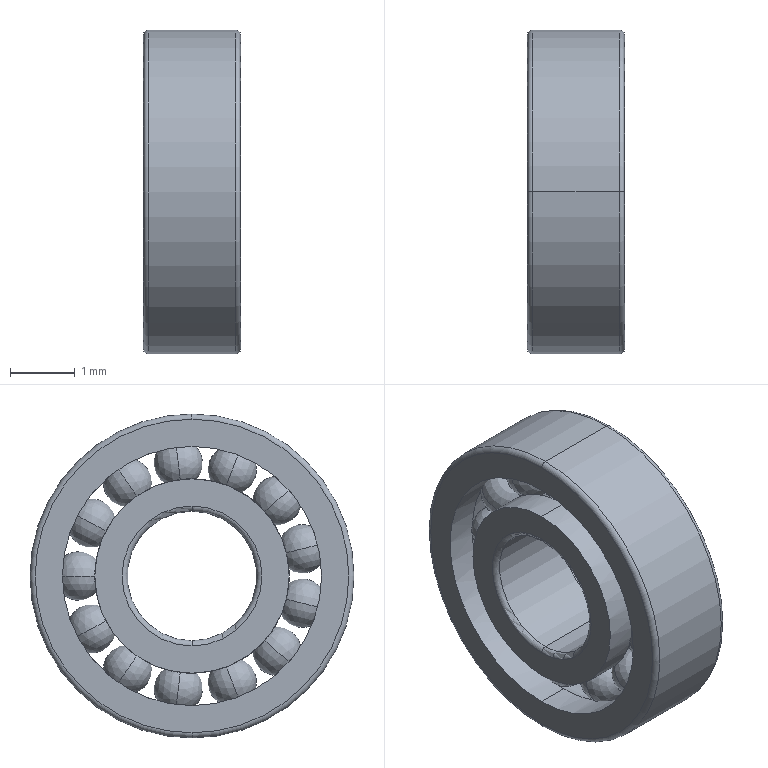Part | SolidWorks | features BaseBody 1 | 1 solid | 92 faces | box 1.5 x 5 x 5 mm | volume 18.357 mm3 | torus 50 | sphere 26 | cylinder 12 | plane 4 | commonest cylinder face diameters 3 x4 4 x4 2 x2 5 x2